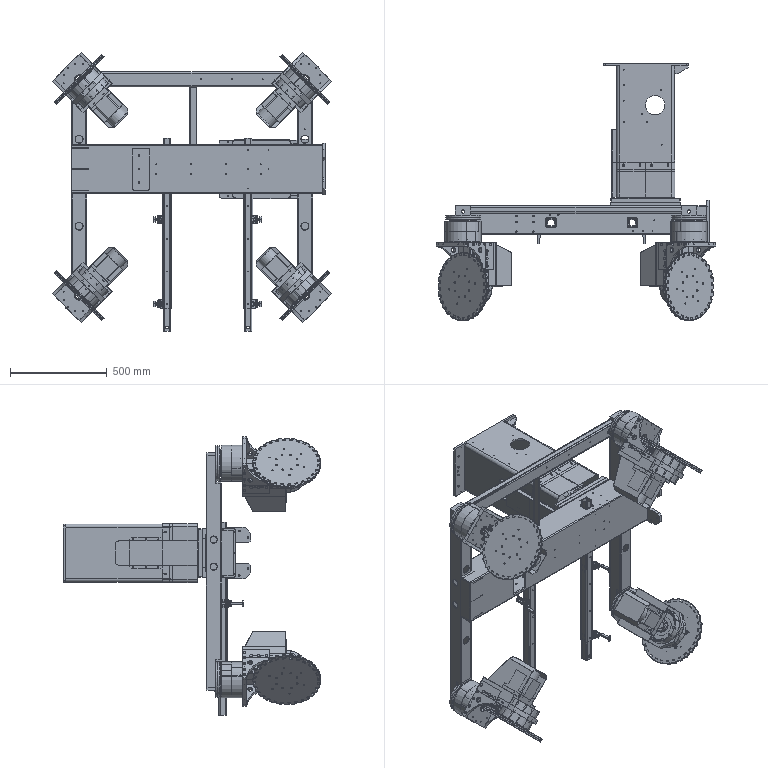Part | SolidWorks | features CompositeCurve 7 | 181 solids | 12957 faces | volume 76260531 mm3 | cylinder 7849 | plane 3437 | cone 1483 | torus 168 | sphere 16 | spline 4 | commonest cylinder face diameters 6 x1334 5 x658 9 x470 6.8 x436 12.5 x432 6.6 x378